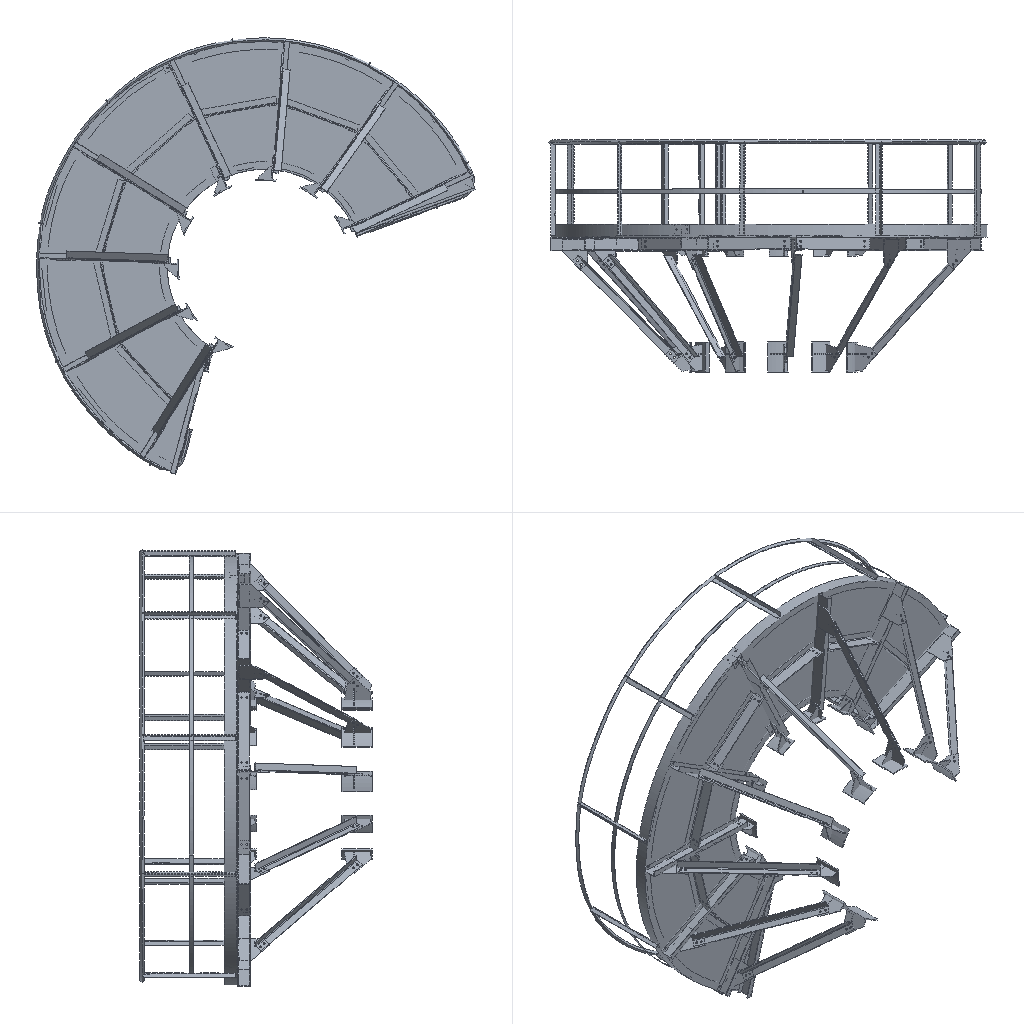Simulation study | ansys workbench
Set-up summary, first 185 of 227 lines:
category,name,step,type,value,unit,region
solver,ansys_workbench
units,mm-N-s-tonne (MPa),,stated,"/units,MPA"
analysis,LS1,,static
load_step,LS1,LS1,static,nsubst=1; time=1
mesh,nodes,,,116393
mesh,elements,,,70113
element_type,SOLID187,,,39621
element_type,TARGE170,,,13795
element_type,CONTA174,,,13795
element_type,SOLID186,,,2782
element_type,SURF154,,,120
material,Structural Steel,,E,200000,tonne s^-2 mm^-1
material,Structural Steel,,nu,0.3
material,Structural Steel,,density,7.85e-09,tonne mm^-3
material,Structural Steel,,conductivity,60.5,tonne mm s^-3 C^-1
material,Structural Steel,,specific_heat,4.34e+08,mm^2 s^-2 C^-1
material,Structural Steel,,cte,1.2e-05,C^-1
material,Structural Steel,,permeability,10000
material,Structural Steel,,resistivity,0.00017,ohm mm
load,Define Force Using Surface Effect Elements,LS1,surface-effect pres face 2,-470.339,,SURF154 #513
bc,Fixed Supports,model,fixed,[dofs=ALL],,_FIXEDSU
contact,Contact Region,,bonded (always),element=CONTA174
contact,Contact Region 2,,bonded (always),element=CONTA174
contact,Contact Region 3,,bonded (always),element=CONTA174
contact,Contact Region 4,,bonded (always),element=CONTA174
contact,Contact Region 5,,bonded (always),element=CONTA174
contact,Contact Region 6,,bonded (always),element=CONTA174
contact,Contact Region 7,,bonded (always),element=CONTA174
contact,Contact Region 8,,bonded (always),element=CONTA174
contact,Contact Region 9,,bonded (always),element=CONTA174
contact,Contact Region 10,,bonded (always),element=CONTA174
contact,Contact Region 11,,bonded (always),element=CONTA174
contact,Contact Region 12,,bonded (always),element=CONTA174
contact,Contact Region 13,,bonded (always),element=CONTA174
contact,Contact Region 14,,bonded (always),element=CONTA174
contact,Contact Region 15,,bonded (always),element=CONTA174
contact,Contact Region 16,,bonded (always),element=CONTA174
contact,Contact Region 17,,bonded (always),element=CONTA174
contact,Contact Region 18,,bonded (always),element=CONTA174
contact,Contact Region 19,,bonded (always),element=CONTA174
contact,Contact Region 20,,bonded (always),element=CONTA174
contact,Contact Region 21,,bonded (always),element=CONTA174
contact,Contact Region 22,,bonded (always),element=CONTA174
contact,Contact Region 23,,bonded (always),element=CONTA174
contact,Contact Region 24,,bonded (always),element=CONTA174
contact,Contact Region 25,,bonded (always),element=CONTA174
contact,Contact Region 26,,bonded (always),element=CONTA174
contact,Contact Region 27,,bonded (always),element=CONTA174
contact,Contact Region 28,,bonded (always),element=CONTA174
contact,Contact Region 29,,bonded (always),element=CONTA174
contact,Contact Region 30,,bonded (always),element=CONTA174
contact,Contact Region 31,,bonded (always),element=CONTA174
contact,Contact Region 32,,bonded (always),element=CONTA174
contact,Contact Region 33,,bonded (always),element=CONTA174
contact,Contact Region 34,,bonded (always),element=CONTA174
contact,Contact Region 35,,bonded (always),element=CONTA174
contact,Contact Region 36,,bonded (always),element=CONTA174
contact,Contact Region 37,,bonded (always),element=CONTA174
contact,Contact Region 38,,bonded (always),element=CONTA174
contact,Contact Region 39,,bonded (always),element=CONTA174
contact,Contact Region 40,,bonded (always),element=CONTA174
contact,Contact Region 41,,bonded (always),element=CONTA174
contact,Contact Region 42,,bonded (always),element=CONTA174
contact,Contact Region 43,,bonded (always),element=CONTA174
contact,Contact Region 44,,bonded (always),element=CONTA174
contact,Contact Region 45,,bonded (always),element=CONTA174
contact,Contact Region 46,,bonded (always),element=CONTA174
contact,Contact Region 47,,bonded (always),element=CONTA174
contact,Contact Region 48,,bonded (always),element=CONTA174
contact,Contact Region 49,,bonded (always),element=CONTA174
contact,Contact Region 50,,bonded (always),element=CONTA174
contact,Contact Region 51,,bonded (always),element=CONTA174
contact,Contact Region 52,,bonded (always),element=CONTA174
contact,Contact Region 53,,bonded (always),element=CONTA174
contact,Contact Region 54,,bonded (always),element=CONTA174
contact,Contact Region 55,,bonded (always),element=CONTA174
contact,Contact Region 56,,bonded (always),element=CONTA174
contact,Contact Region 57,,bonded (always),element=CONTA174
contact,Contact Region 58,,bonded (always),element=CONTA174
contact,Contact Region 59,,bonded (always),element=CONTA174
contact,Contact Region 60,,bonded (always),element=CONTA174
contact,Contact Region 61,,bonded (always),element=CONTA174
contact,Contact Region 62,,bonded (always),element=CONTA174
contact,Contact Region 63,,bonded (always),element=CONTA174
contact,Contact Region 64,,bonded (always),element=CONTA174
contact,Contact Region 65,,bonded (always),element=CONTA174
contact,Contact Region 66,,bonded (always),element=CONTA174
contact,Contact Region 67,,bonded (always),element=CONTA174
contact,Contact Region 68,,bonded (always),element=CONTA174
contact,Contact Region 69,,bonded (always),element=CONTA174
contact,Contact Region 70,,bonded (always),element=CONTA174
contact,Contact Region 71,,bonded (always),element=CONTA174
contact,Contact Region 72,,bonded (always),element=CONTA174
contact,Contact Region 73,,bonded (always),element=CONTA174
contact,Contact Region 74,,bonded (always),element=CONTA174
contact,Contact Region 75,,bonded (always),element=CONTA174
contact,Contact Region 76,,bonded (always),element=CONTA174
contact,Contact Region 77,,bonded (always),element=CONTA174
contact,Contact Region 78,,bonded (always),element=CONTA174
contact,Contact Region 79,,bonded (always),element=CONTA174
contact,Contact Region 80,,bonded (always),element=CONTA174
contact,Contact Region 81,,bonded (always),element=CONTA174
contact,Contact Region 82,,bonded (always),element=CONTA174
contact,Contact Region 83,,bonded (always),element=CONTA174
contact,Contact Region 84,,bonded (always),element=CONTA174
contact,Contact Region 85,,bonded (always),element=CONTA174
contact,Contact Region 86,,bonded (always),element=CONTA174
contact,Contact Region 87,,bonded (always),element=CONTA174
contact,Contact Region 88,,bonded (always),element=CONTA174
contact,Contact Region 89,,bonded (always),element=CONTA174
contact,Contact Region 90,,bonded (always),element=CONTA174
contact,Contact Region 91,,bonded (always),element=CONTA174
contact,Contact Region 92,,bonded (always),element=CONTA174
contact,Contact Region 93,,bonded (always),element=CONTA174
contact,Contact Region 94,,bonded (always),element=CONTA174
contact,Contact Region 95,,bonded (always),element=CONTA174
contact,Contact Region 96,,bonded (always),element=CONTA174
contact,Contact Region 97,,bonded (always),element=CONTA174
contact,Contact Region 98,,bonded (always),element=CONTA174
contact,Contact Region 99,,bonded (always),element=CONTA174
contact,Contact Region 100,,bonded (always),element=CONTA174
contact,Contact Region 101,,bonded (always),element=CONTA174
contact,Contact Region 102,,bonded (always),element=CONTA174
contact,Contact Region 103,,bonded (always),element=CONTA174
contact,Contact Region 104,,bonded (always),element=CONTA174
contact,Contact Region 105,,bonded (always),element=CONTA174
contact,Contact Region 106,,bonded (always),element=CONTA174
contact,Contact Region 107,,bonded (always),element=CONTA174
contact,Contact Region 108,,bonded (always),element=CONTA174
contact,Contact Region 109,,bonded (always),element=CONTA174
contact,Contact Region 110,,bonded (always),element=CONTA174
contact,Contact Region 111,,bonded (always),element=CONTA174
contact,Contact Region 112,,bonded (always),element=CONTA174
contact,Contact Region 113,,bonded (always),element=CONTA174
contact,Contact Region 114,,bonded (always),element=CONTA174
contact,Contact Region 115,,bonded (always),element=CONTA174
contact,Contact Region 116,,bonded (always),element=CONTA174
contact,Contact Region 117,,bonded (always),element=CONTA174
contact,Contact Region 118,,bonded (always),element=CONTA174
contact,Contact Region 119,,bonded (always),element=CONTA174
contact,Contact Region 120,,bonded (always),element=CONTA174
contact,Contact Region 121,,bonded (always),element=CONTA174
contact,Contact Region 122,,bonded (always),element=CONTA174
contact,Contact Region 123,,bonded (always),element=CONTA174
contact,Contact Region 124,,bonded (always),element=CONTA174
contact,Contact Region 125,,bonded (always),element=CONTA174
contact,Contact Region 126,,bonded (always),element=CONTA174
contact,Contact Region 127,,bonded (always),element=CONTA174
contact,Contact Region 128,,bonded (always),element=CONTA174
contact,Contact Region 129,,bonded (always),element=CONTA174
contact,Contact Region 130,,bonded (always),element=CONTA174
contact,Contact Region 131,,bonded (always),element=CONTA174
contact,Contact Region 132,,bonded (always),element=CONTA174
contact,Contact Region 133,,bonded (always),element=CONTA174
contact,Contact Region 134,,bonded (always),element=CONTA174
contact,Contact Region 135,,bonded (always),element=CONTA174
contact,Contact Region 136,,bonded (always),element=CONTA174
contact,Contact Region 137,,bonded (always),element=CONTA174
contact,Contact Region 138,,bonded (always),element=CONTA174
contact,Contact Region 139,,bonded (always),element=CONTA174
contact,Contact Region 140,,bonded (always),element=CONTA174
contact,Contact Region 141,,bonded (always),element=CONTA174
contact,Contact Region 142,,bonded (always),element=CONTA174
contact,Contact Region 143,,bonded (always),element=CONTA174
contact,Contact Region 144,,bonded (always),element=CONTA174
contact,Contact Region 145,,bonded (always),element=CONTA174
contact,Contact Region 146,,bonded (always),element=CONTA174
contact,Contact Region 147,,bonded (always),element=CONTA174
contact,Contact Region 148,,bonded (always),element=CONTA174
contact,Contact Region 149,,bonded (always),element=CONTA174
contact,Contact Region 150,,bonded (always),element=CONTA174
contact,Contact Region 151,,bonded (always),element=CONTA174
contact,Contact Region 152,,bonded (always),element=CONTA174
contact,Contact Region 153,,bonded (always),element=CONTA174
contact,Contact Region 154,,bonded (always),element=CONTA174
contact,Contact Region 155,,bonded (always),element=CONTA174
contact,Contact Region 156,,bonded (always),element=CONTA174
contact,Contact Region 157,,bonded (always),element=CONTA174
contact,Contact Region 158,,bonded (always),element=CONTA174
contact,Contact Region 159,,bonded (always),element=CONTA174
contact,Contact Region 160,,bonded (always),element=CONTA174
contact,Contact Region 161,,bonded (always),element=CONTA174
contact,Contact Region 162,,bonded (always),element=CONTA174
contact,Contact Region 163,,bonded (always),element=CONTA174
Ansys APDL input file, long lists of numbers shortened:
/batch
/config,noeldb,1     ! force off writing results to database
*get,_wallstrt,active,,time,wall
! ANSYS input file written by Workbench version 2022 R1
! File used for geometry attach:
/title,wbnew--____ (B5)
! ****** Begin Custom Load Command Snippet ******
/COM, ACT Extensions:
/COM,     LSDYNA, 2021.1
/COM,
! ****** End   Custom Load Command Snippet ******
*DIM,_wb_ProjectScratch_dir,string,248
_wb_ProjectScratch_dir(1) = ''
*DIM,_wb_SolverFiles_dir,string,248
_wb_SolverFiles_dir(1) = ''
*DIM,_wb_userfiles_dir,string,248
_wb_userfiles_dir(1) = ''
/com,--- Data in consistent NMM units. See Solving Units in the help system for more information.
/units,MPA
/nopr
/wb,file,start              !  signify a WB generated input file
/prep7
! Turn off shape checking because checks already performed inside WB mesher.
! See help system for more information.
SHPP,OFF,,NOWARN
/nolist
etcon,set             ! allow ANSYS to choose best KEYOP's for 180x elements, resets any applicable keyopt to MAPDL defaults
/com,*********** Nodes for the whole assembly ***********
nblock,3,,128032
(1i9,3e20.9e3)
        1    -3.929116873E+02    -2.210244133E+02    -9.488822832E+02
! (116392 more lines like these left out)
-1
/wb,elem,start            !  set before creation of elements
/com,*********** Elements for Body 1 "VZ33-01-10_ASM|VZ33-01-11____160-65X8|VZ33-01-11____160-65X8[1]" ***********
et,1,187
eblock,19,solid,,978
(19i9)
        1        1        1        1        0        0        0        0       10        0    27157    79887    80024    79897    79888    80427    80471    80423    80419
! (1955 more lines like these left out)
-1
/com,*********** Elements for Body 2 "VZ33-01-10_ASM|VZ33-01-15____10|VZ33-01-15____10[1]" ***********
et,2,186
keyo,2,2,1          ! set full integration on SOLID186
eblock,19,solid,,56
(19i9)
        2        2        2        2        0        0        0        0       20        0      309     2559     2562     2661     2592     2630     2627     2698     2597
! (111 more lines like these left out)
-1
/com,*********** Elements for Body 3 "VZ33-01-10_ASM|VZ33-01-12____100X100X10|VZ33-01-12____100X100X10[1]" ***********
et,3,187
eblock,19,solid,,504
(19i9)
        3        3        3        3        0        0        0        0       10        0    13418    47156    47216    47205    47250    47537    47849    47536    47539
! (1007 more lines like these left out)
-1
/com,*********** Elements for Body 4 "VZ33-01-10_ASM|VZ33-01-14____10|VZ33-01-14____10[1]" ***********
et,4,187
eblock,19,solid,,460
(19i9)
        4        4        4        4        0        0        0        0       10        0     3210    13522    13559    13549    13576    14313    14428    14312    14314
! (919 more lines like these left out)
-1
/com,*********** Elements for Body 5 "VZ33-01-10_ASM|VZ33-01-18____16|VZ33-01-18____16[1]" ***********
et,5,186
keyo,5,2,1          ! set full integration on SOLID186
eblock,19,solid,,70
(19i9)
        5        5        5        5        0        0        0        0       20        0      365     3121     3194     3209     3142     3125     3195     3196     3126
! (139 more lines like these left out)
-1
! (99 more sections like these left out)
/wb,elem,end               !  done creating elements
/com,*********** Send User Defined Coordinate System(s) ***********
csys,0
toffst,273.15,  ! Temperature offset from absolute zero
/com,*********** Set Reference Temperature ***********
tref,22.
/wb,mat,start              !  starting to send materials
/com,*********** Send Materials ***********
Temperature = 'TEMP' ! Temperature
MP,DENS,1,7.85e-09,	! tonne mm^-3
MP,ALPX,1,1.2e-05,	! C^-1
MP,C,1,434000000,	! mm^2 s^-2 C^-1
MP,KXX,1,60.5,	! tonne mm s^-3 C^-1
MP,RSVX,1,0.00017,	! ohm mm
MP,EX,1,200000,	! tonne s^-2 mm^-1
MP,NUXY,1,0.3,
MP,MURX,1,10000,
Temperature = 'TEMP' ! Temperature
MP,DENS,2,7.85e-09,	! tonne mm^-3
MP,ALPX,2,1.2e-05,	! C^-1
MP,C,2,434000000,	! mm^2 s^-2 C^-1
MP,KXX,2,60.5,	! tonne mm s^-3 C^-1
MP,RSVX,2,0.00017,	! ohm mm
MP,EX,2,200000,	! tonne s^-2 mm^-1
MP,NUXY,2,0.3,
MP,MURX,2,10000,
Temperature = 'TEMP' ! Temperature
MP,DENS,3,7.85e-09,	! tonne mm^-3
MP,ALPX,3,1.2e-05,	! C^-1
MP,C,3,434000000,	! mm^2 s^-2 C^-1
MP,KXX,3,60.5,	! tonne mm s^-3 C^-1
MP,RSVX,3,0.00017,	! ohm mm
MP,EX,3,200000,	! tonne s^-2 mm^-1
MP,NUXY,3,0.3,
MP,MURX,3,10000,
Temperature = 'TEMP' ! Temperature
MP,DENS,4,7.85e-09,	! tonne mm^-3
MP,ALPX,4,1.2e-05,	! C^-1
MP,C,4,434000000,	! mm^2 s^-2 C^-1
MP,KXX,4,60.5,	! tonne mm s^-3 C^-1
MP,RSVX,4,0.00017,	! ohm mm
MP,EX,4,200000,	! tonne s^-2 mm^-1
MP,NUXY,4,0.3,
MP,MURX,4,10000,
Temperature = 'TEMP' ! Temperature
MP,DENS,5,7.85e-09,	! tonne mm^-3
MP,ALPX,5,1.2e-05,	! C^-1
MP,C,5,434000000,	! mm^2 s^-2 C^-1
MP,KXX,5,60.5,	! tonne mm s^-3 C^-1
MP,RSVX,5,0.00017,	! ohm mm
MP,EX,5,200000,	! tonne s^-2 mm^-1
MP,NUXY,5,0.3,
MP,MURX,5,10000,
Temperature = 'TEMP' ! Temperature
MP,DENS,6,7.85e-09,	! tonne mm^-3
MP,ALPX,6,1.2e-05,	! C^-1
MP,C,6,434000000,	! mm^2 s^-2 C^-1
MP,KXX,6,60.5,	! tonne mm s^-3 C^-1
MP,RSVX,6,0.00017,	! ohm mm
MP,EX,6,200000,	! tonne s^-2 mm^-1
MP,NUXY,6,0.3,
MP,MURX,6,10000,
Temperature = 'TEMP' ! Temperature
MP,DENS,7,7.85e-09,	! tonne mm^-3
MP,ALPX,7,1.2e-05,	! C^-1
MP,C,7,434000000,	! mm^2 s^-2 C^-1
MP,KXX,7,60.5,	! tonne mm s^-3 C^-1
MP,RSVX,7,0.00017,	! ohm mm
MP,EX,7,200000,	! tonne s^-2 mm^-1
MP,NUXY,7,0.3,
MP,MURX,7,10000,
Temperature = 'TEMP' ! Temperature
MP,DENS,8,7.85e-09,	! tonne mm^-3
MP,ALPX,8,1.2e-05,	! C^-1
MP,C,8,434000000,	! mm^2 s^-2 C^-1
MP,KXX,8,60.5,	! tonne mm s^-3 C^-1
MP,RSVX,8,0.00017,	! ohm mm
MP,EX,8,200000,	! tonne s^-2 mm^-1
MP,NUXY,8,0.3,
MP,MURX,8,10000,
Temperature = 'TEMP' ! Temperature
MP,DENS,9,7.85e-09,	! tonne mm^-3
MP,ALPX,9,1.2e-05,	! C^-1
MP,C,9,434000000,	! mm^2 s^-2 C^-1
MP,KXX,9,60.5,	! tonne mm s^-3 C^-1
MP,RSVX,9,0.00017,	! ohm mm
MP,EX,9,200000,	! tonne s^-2 mm^-1
! (857 more lines like these left out)
/wb,mat,end                !  done sending materials
!************************* Model Summary ********************
!VZ33-01-10_ASM|VZ33-01-11____160-65X8|VZ33-01-11____160-65X8[1],	结构钢,	matid,	1
!VZ33-01-10_ASM|VZ33-01-15____10|VZ33-01-15____10[1],	结构钢,	matid,	2
!VZ33-01-10_ASM|VZ33-01-12____100X100X10|VZ33-01-12____100X100X10[1],	结构钢,	matid,	3
! (103 more lines like these left out)
*get,_xmin,node,,mnloc,x
*get,_ymin,node,,mnloc,y
*get,_zmin,node,,mnloc,z
*get,_xmax,node,,mxloc,x
*get,_ymax,node,,mxloc,y
*get,_zmax,node,,mxloc,z
_ASMDIAG=(_xmax-_xmin)*(_xmax-_xmin)+(_ymax-_ymin)*(_ymax-_ymin)+(_zmax-_zmin)*(_zmax-_zmin)
_ASMDIAG=SQRT(_ASMDIAG)
/wb,contact,start          !  starting to send contact
/com,*********** Create Contact "接触区域" ***********
/com,            Real Constant Set For Above Contact Is 106 & 105
*set,tid,106
*set,cid,105
r,tid
r,cid
et,tid,170
et,cid,174
eblock,10,,,13
(15i9)
    84676      106      106      106        0    79927    80031    79937    79937    80706    80825    79937    80704
! (12 more lines like these left out)
-1
eblock,10,,,13
(15i9)
    84689      105      105      105        0    79927    80031    79937    79937    80706    80825    79937    80704
! (12 more lines like these left out)
-1
eblock,10,,,28
(15i9)
    84702      105      106      105        0     2643     2571     2594     2644     2758     2756     2826     2940
! (27 more lines like these left out)
-1
eblock,10,,,28
(15i9)
    84730      106      105      106        0     2643     2571     2594     2644     2758     2756     2826     2940
! (27 more lines like these left out)
-1
keyo,cid,8,2               ! auto create asymmetric contact (from Program Controlled setting)
keyo,cid,10,0              ! adjust contact stiffness each NR iteration (from Program Controlled setting)
keyo,cid,12,5              ! bonded always
keyo,cid,18,1              ! small sliding turned on by application
keyo,cid,2,0               ! augmented Lagrange (from Program Controlled setting)
keyo,cid,4,0               ! on Gauss point (from Program Controlled setting)
keyo,cid,9,1               ! ignore initial gaps/penetration
keyo,cid,7,0               ! No Prediction
rmod,tid,3,10.      ! FKN
rmod,tid,5,0.       ! ICONT
rmod,tid,6,0.       ! PINB
rmod,tid,10,0.      ! CNOF
rmod,tid,12,0.      ! FKT
rmod,tid,36,335     ! WB DSID
rmod,cid,3,10.      ! FKN
rmod,cid,5,0.       ! ICONT
rmod,cid,6,0.       ! PINB
rmod,cid,10,0.      ! CNOF
rmod,cid,12,0.      ! FKT
rmod,cid,36,335     ! WB DSID
/com,*********** Create Contact "接触区域 2" ***********
/com,            Real Constant Set For Above Contact Is 108 & 107
*set,tid,108
*set,cid,107
r,tid
r,cid
et,tid,170
et,cid,174
eblock,10,,,28
(15i9)
    84758      108      108      108        0    79863    79871    80025    80025    80302    80346    80025    80306
! (27 more lines like these left out)
-1
eblock,10,,,28
(15i9)
    84786      107      107      107        0    79863    79871    80025    80025    80302    80346    80025    80306
! (27 more lines like these left out)
-1
eblock,10,,,79
(15i9)
    84814      107      108      107        0    14634    14637    14642    14642    15440    15457    14642    15441
! (78 more lines like these left out)
-1
eblock,10,,,79
(15i9)
    84893      108      107      108        0    14634    14637    14642    14642    15440    15457    14642    15441
! (78 more lines like these left out)
-1
keyo,cid,8,2               ! auto create asymmetric contact (from Program Controlled setting)
keyo,cid,10,0              ! adjust contact stiffness each NR iteration (from Program Controlled setting)
keyo,cid,12,5              ! bonded always
keyo,cid,18,1              ! small sliding turned on by application
keyo,cid,2,0               ! augmented Lagrange (from Program Controlled setting)
keyo,cid,4,0               ! on Gauss point (from Program Controlled setting)
keyo,cid,9,1               ! ignore initial gaps/penetration
keyo,cid,7,0               ! No Prediction
rmod,tid,3,10.      ! FKN
rmod,tid,5,0.       ! ICONT
rmod,tid,6,0.       ! PINB
rmod,tid,10,0.      ! CNOF
rmod,tid,12,0.      ! FKT
rmod,tid,36,338     ! WB DSID
rmod,cid,3,10.      ! FKN
rmod,cid,5,0.       ! ICONT
rmod,cid,6,0.       ! PINB
rmod,cid,10,0.      ! CNOF
rmod,cid,12,0.      ! FKT
rmod,cid,36,338     ! WB DSID
/com,*********** Create Contact "接触区域 3" ***********
/com,            Real Constant Set For Above Contact Is 110 & 109
*set,tid,110
*set,cid,109
r,tid
r,cid
et,tid,170
et,cid,174
eblock,10,,,7
(15i9)
    84972      110      110      110        0    79936    80030    80043    80043    80814    81397    80043    80815
! (6 more lines like these left out)
-1
eblock,10,,,7
(15i9)
    84979      109      109      109        0    79936    80030    80043    80043    80814    81397    80043    80815
! (6 more lines like these left out)
-1
eblock,10,,,19
(15i9)
    84986      109      110      109        0    22203    22280    22323    22323    22855    23186    22323    22857
! (18 more lines like these left out)
-1
eblock,10,,,19
(15i9)
    85005      110      109      110        0    22203    22280    22323    22323    22855    23186    22323    22857
! (18 more lines like these left out)
-1
keyo,cid,8,2               ! auto create asymmetric contact (from Program Controlled setting)
keyo,cid,10,0              ! adjust contact stiffness each NR iteration (from Program Controlled setting)
keyo,cid,12,5              ! bonded always
keyo,cid,18,1              ! small sliding turned on by application
keyo,cid,2,0               ! augmented Lagrange (from Program Controlled setting)
keyo,cid,4,0               ! on Gauss point (from Program Controlled setting)
keyo,cid,9,1               ! ignore initial gaps/penetration
keyo,cid,7,0               ! No Prediction
rmod,tid,3,10.      ! FKN
rmod,tid,5,0.       ! ICONT
rmod,tid,6,0.       ! PINB
rmod,tid,10,0.      ! CNOF
rmod,tid,12,0.      ! FKT
rmod,tid,36,341     ! WB DSID
rmod,cid,3,10.      ! FKN
rmod,cid,5,0.       ! ICONT
rmod,cid,6,0.       ! PINB
rmod,cid,10,0.      ! CNOF
rmod,cid,12,0.      ! FKT
rmod,cid,36,341     ! WB DSID
/com,*********** Create Contact "接触区域 4" ***********
/com,            Real Constant Set For Above Contact Is 112 & 111
*set,tid,112
*set,cid,111
r,tid
r,cid
et,tid,170
et,cid,174
eblock,10,,,5
(15i9)
    85024      112      112      112        0    80029    79924    80042    80042    80668    80669    80042    81389
    85025      112      112      112        0    80043    79925    79935    79935    80682    80676    79935    80806
    85026      112      112      112        0    79935    80029    80042    80042    80804    81389    80042    80805
    85027      112      112      112        0    79925    80029    79935    79935    80680    80804    79935    80676
    85028      112      112      112        0    80042    79924    79934    79934    80669    80662    79934    80794
-1
eblock,10,,,5
(15i9)
    85029      111      111      111        0    80029    79924    80042    80042    80668    80669    80042    81389
    85030      111      111      111        0    80043    79925    79935    79935    80682    80676    79935    80806
    85031      111      111      111        0    79935    80029    80042    80042    80804    81389    80042    80805
    85032      111      111      111        0    79925    80029    79935    79935    80680    80804    79935    80676
    85033      111      111      111        0    80042    79924    79934    79934    80669    80662    79934    80794
-1
eblock,10,,,7
(15i9)
    85034      111      112      111        0    27934    27897    27898    27933    28124    28123    28126    28182
! (6 more lines like these left out)
-1
eblock,10,,,7
(15i9)
    85041      112      111      112        0    27934    27897    27898    27933    28124    28123    28126    28182
! (6 more lines like these left out)
-1
keyo,cid,8,2               ! auto create asymmetric contact (from Program Controlled setting)
keyo,cid,10,0              ! adjust contact stiffness each NR iteration (from Program Controlled setting)
keyo,cid,12,5              ! bonded always
keyo,cid,18,1              ! small sliding turned on by application
keyo,cid,2,0               ! augmented Lagrange (from Program Controlled setting)
keyo,cid,4,0               ! on Gauss point (from Program Controlled setting)
keyo,cid,9,1               ! ignore initial gaps/penetration
keyo,cid,7,0               ! No Prediction
rmod,tid,3,10.      ! FKN
rmod,tid,5,0.       ! ICONT
rmod,tid,6,0.       ! PINB
rmod,tid,10,0.      ! CNOF
rmod,tid,12,0.      ! FKT
rmod,tid,36,344     ! WB DSID
rmod,cid,3,10.      ! FKN
rmod,cid,5,0.       ! ICONT
rmod,cid,6,0.       ! PINB
rmod,cid,10,0.      ! CNOF
rmod,cid,12,0.      ! FKT
rmod,cid,36,344     ! WB DSID
/com,*********** Create Contact "接触区域 5" ***********
/com,            Real Constant Set For Above Contact Is 114 & 113
*set,tid,114
*set,cid,113
r,tid
r,cid
et,tid,170
et,cid,174
eblock,10,,,82
(15i9)
    85048      114      114      114        0    80009    80030    79906    79906    81309    80537    79906    80534
! (81 more lines like these left out)
-1
eblock,10,,,82
(15i9)
    85130      113      113      113        0    80009    80030    79906    79906    81309    80537    79906    80534
! (81 more lines like these left out)
-1
eblock,10,,,9
(15i9)
    85212      113      114      113        0    95158    95071    95160    95159    95328    95329    95509    95508
! (8 more lines like these left out)
-1
eblock,10,,,9
(15i9)
    85221      114      113      114        0    95158    95071    95160    95159    95328    95329    95509    95508
! (8 more lines like these left out)
-1
keyo,cid,8,2               ! auto create asymmetric contact (from Program Controlled setting)
keyo,cid,10,0              ! adjust contact stiffness each NR iteration (from Program Controlled setting)
keyo,cid,12,5              ! bonded always
keyo,cid,18,1              ! small sliding turned on by application
keyo,cid,2,0               ! augmented Lagrange (from Program Controlled setting)
keyo,cid,4,0               ! on Gauss point (from Program Controlled setting)
keyo,cid,9,1               ! ignore initial gaps/penetration
keyo,cid,7,0               ! No Prediction
rmod,tid,3,10.      ! FKN
rmod,tid,5,0.       ! ICONT
rmod,tid,6,0.       ! PINB
rmod,tid,10,0.      ! CNOF
rmod,tid,12,0.      ! FKT
rmod,tid,36,347     ! WB DSID
rmod,cid,3,10.      ! FKN
rmod,cid,5,0.       ! ICONT
rmod,cid,6,0.       ! PINB
rmod,cid,10,0.      ! CNOF
rmod,cid,12,0.      ! FKT
rmod,cid,36,347     ! WB DSID
! (199 more sections like these left out)
/wb,contact,end            !  done creating contacts
/golist
/wb,load,start             !  starting to send loads
/com,*********** Fixed Supports ***********
CMBLOCK,_FIXEDSU,NODE,    91196
(8i10)
         1         2         3         4         5         6         7         8
! (11399 more lines like these left out)
cmsel,s,_FIXEDSU
d,all,all
nsel,all
/com,*********** Define Force Using Surface Effect Elements ***********
local,12,0,0.,0.,0.,0.,0.,0.
csys,0
et,513,154
eblock,10,,,120
(15i9)
   112266      513      513      513       12    96640    96561    96670    96641    96819    96820    96994    96992
! (119 more lines like these left out)
-1
esel,s,type,,513
keyop,513,2,1                ! Apply load in local coordinate system
keyop,513,7,1                ! Use original area so load is constant in large deformation
esel,all
/gst,on,on
fini
*get,_numnode,node,0,count
*get,_numelem,elem,0,count
*get, _MAXELEMNUM, elem, 0, NUM, MAX
*get, _MAXNODENUM, node, 0, NUM, MAX
*get, _MAXELEMTYPE, etyp, 0, NUM, MAX
*get, _MAXREALCONST, real, 0, NUM, MAX
/go
/wb,load,end               !  done creating loads
/com,--- Number of total nodes = %_numnode%
/com,--- Number of contact elements = 27710
/com,--- Number of spring elements = 0
/com,--- Number of bearing elements = 0
/com,--- Number of solid elements = 42403
/com,--- Number of condensed parts = 0
/com,--- Number of total elements = %_numelem%
*get,_wallbsol,active,,time,wall
/com,****************************************************************************
/com,*************************    SOLUTION       ********************************
/com,****************************************************************************
/solu
antype,0                   ! static analysis
_thickRatio=0.00962 ! Ratio of thick parts in the model
eqsl,sparse,,,,,1
cntr,print,1               ! print out contact info and also make no initial contact an error
cntr,out,yes               ! write contact output to file.cmn due to many contact pairs present
dmpoption,emat,no             ! Don't combine emat file for DANSYS
dmpoption,esav,no             ! Don't combine esav file for DANSYS
nldiag,cont,iter           ! print out contact info each equilibrium iteration
rescontrol,,none                 ! Do not keep any restart files
/com,****************************************************
/com,******************* SOLVE FOR LS 1 OF 1 ****************
esel,s,type,,513
nsle
sfe,all,1,pres,1,0.
sfe,all,2,pres,1,-470.339
sfe,all,3,pres,1,0.
nsel,all
esel,all
/nopr
/gopr
nsub,1,1,1
time,1.
outres,erase
outres,all,none
outres,nsol,all,
outres,rsol,all
outres,eangl,all
outres,etmp,all
outres,veng,all
outres,strs,all,
outres,epel,all,
outres,eppl,all,
outres,cont,all,
! *********** WB SOLVE COMMAND ***********
! check interactive state
*get,ANSINTER_,active,,int
*if,ANSINTER_,ne,0,then
/eof
*endif
solve
/com *************** Write FE CONNECTORS *********
CEWRITE,file,ce,,INTE
/com,****************************************************
/com,*************** FINISHED SOLVE FOR LS 1 *************
*get,_wallasol,active,,time,wall
/nopr
*get,_numnode,node,0,count
*get,_numelem,elem,0,count
*get, _MAXELEMNUM, elem, 0, NUM, MAX
*get, _MAXNODENUM, node, 0, NUM, MAX,,,INTERNAL
*get, _MAXELEMTYPE, etyp, 0, NUM, MAX
*get, _MAXREALCONST, real, 0, NUM, MAX
/gopr
/post1
xmlo,ENCODING,ISO-8859-1
xmlo,parm
/xml,parm,xml
fini
/gopr
*get,_walldone,active,,time,wall
_preptime=(_wallbsol-_wallstrt)*3600
_solvtime=(_wallasol-_wallbsol)*3600
_posttime=(_walldone-_wallasol)*3600
_totaltim=(_walldone-_wallstrt)*3600
*get,_dlbratio,active,0,solu,dlbr
*get,_combtime,active,0,solu,comb
*get,_ssmode,active,0,solu,ssmm
*get,_ndofs,active,0,solu,ndof
*get,_sol_end_time,active,0,set,time
*if,_sol_end_time,eq,1.,then
/fclean				!clean distributed files
*endif
/com,--- Total number of nodes = %_numnode%
/com,--- Total number of elements = %_numelem%
/com,--- Element load balance ratio = %_dlbratio%
/com,--- Time to combine distributed files = %_combtime%
/com,--- Sparse memory mode = %_ssmode%
/com,--- Number of DOF = %_ndofs%
/wb,file,end               ! done with WB generated input
Results summary:
result,analyses[0].index,,,1
result,analyses[0].system,,,SYS
result,analyses[0].deck,,,deck.dat
result,analyses[0].solve_status,,,completed
result,analyses[0].analysis_type,,,static
result,analyses[0].physics,,,mechanical
result,analyses[0].unit_system,,,"NMM: mm, ton, N, s, mV, mA, degC"
result,analyses[0].n_sets,,,1
result,analyses[0].load_steps[0].set,set=1,,1
result,analyses[0].load_steps[0].time_or_freq,set=1,,1
result,analyses[0].load_steps[0].max_displacement_magnitude,set=1,,0.1432
result,analyses[0].load_steps[0].max_von_mises_nodal,set=1,,488.954
result,analyses[0].load_steps[0].reaction_force_sum_xyz[1],set=1,,3.49109e-08
result,analyses[0].load_steps[0].reaction_force_sum_xyz[2],set=1,,5e+09
result,analyses[0].load_steps[0].reaction_force_sum_xyz[3],set=1,,3.92765e-08